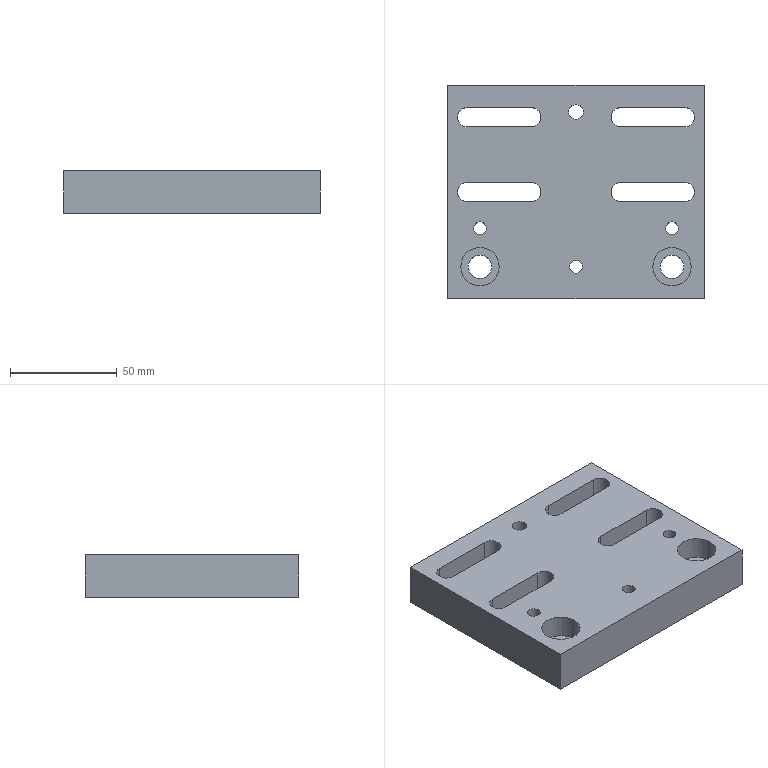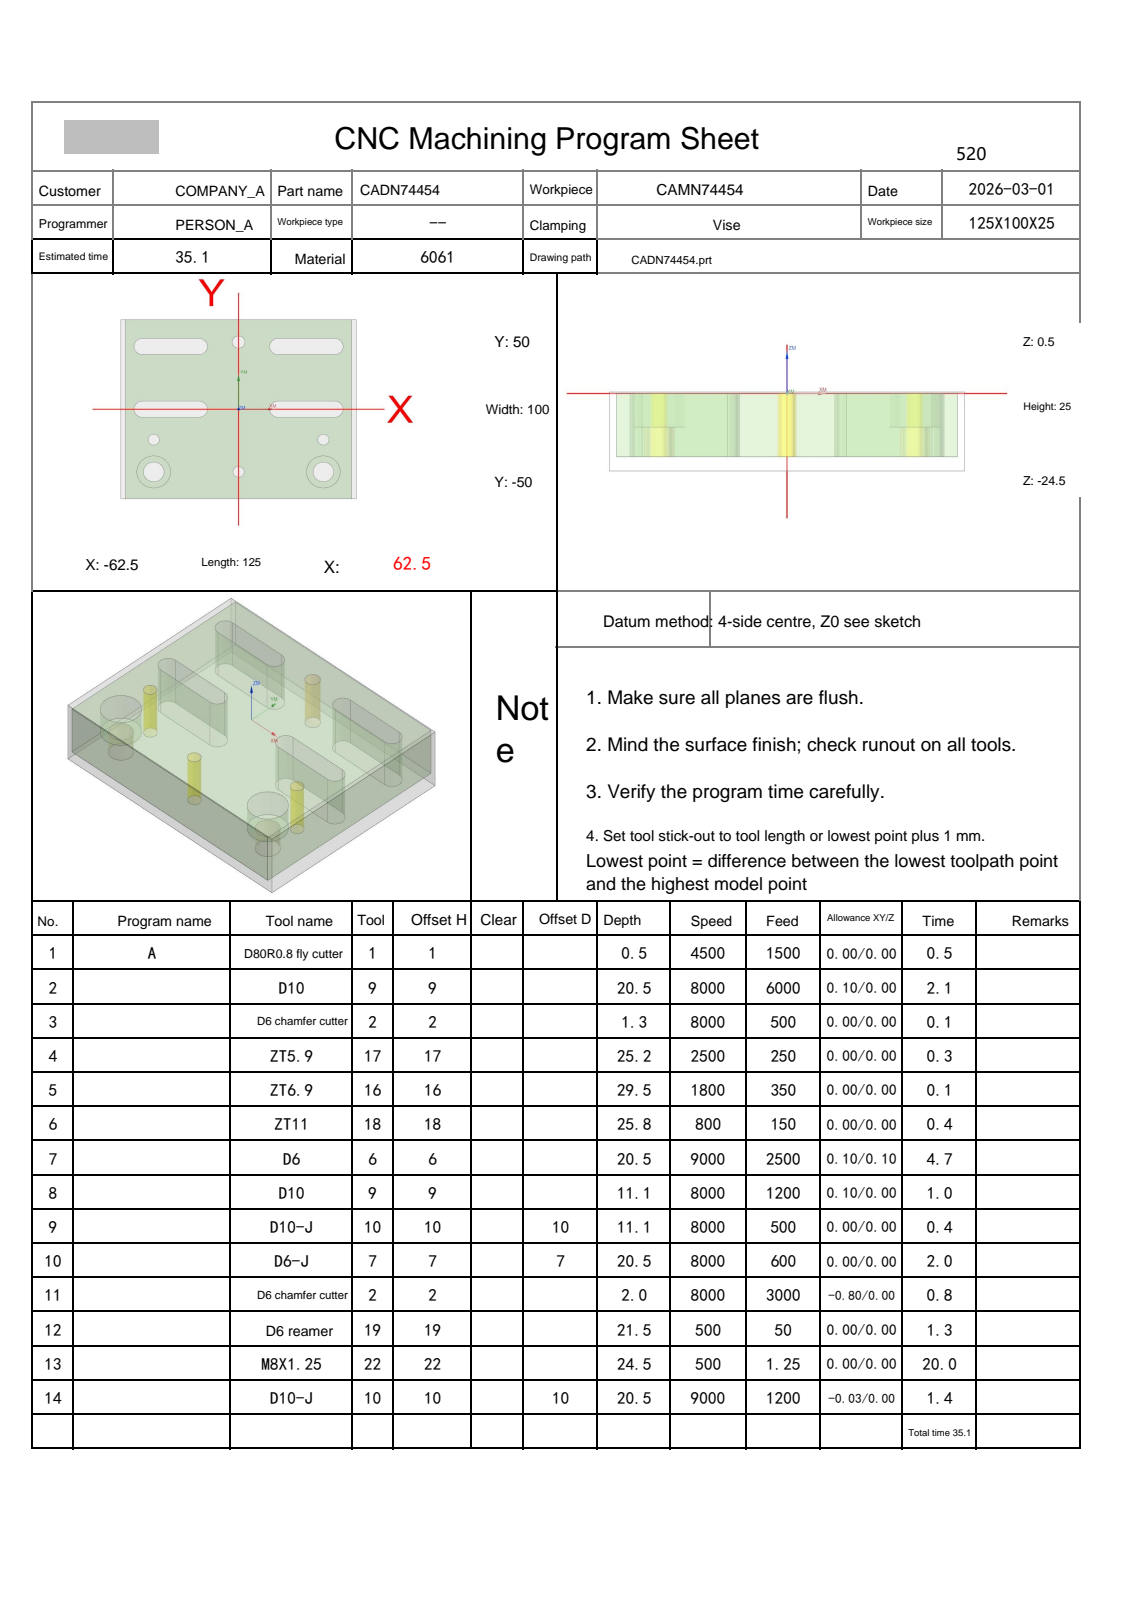NC program | NX | posted by the shop | part box 120 x 100 x 20 mm
Lines 2070 to 2160 of 2160:
N14 T10 M06
(D10-J  D=10. R=0. H=10 ce=0.00 di=0.00)
G00 G90 G54 X-61.013 Y56.116 M03 S9000
G43 H10 Z50.
M08
Z-9.5
G01 Z-10. F1200.
G41 D10
X-60.997 Y55.917
G03 X-60. Y55. I.997 J.083
G01 X60.
G02 X65. Y50. I0.0 J-5.
G01 Y-50.
G02 X60. Y-55. I-5. J0.0
G01 X-60.
G02 X-65. Y-50. I0.0 J5.
G01 Y50.
G02 X-60. Y55. I5. J0.0
G01 X-59.5
G03 X-58.5 Y56. I0.0 J1.
G01 G40 Y56.2
Z-9.5
G00 Z50.
X-61.013 Y56.116
Z-19.5
G01 Z-20.
G41 D10
X-60.997 Y55.917
G03 X-60. Y55. I.997 J.083
G01 X60.
G02 X65. Y50. I0.0 J-5.
G01 Y-50.
G02 X60. Y-55. I-5. J0.0
G01 X-60.
G02 X-65. Y-50. I0.0 J5.
G01 Y50.
G02 X-60. Y55. I5. J0.0
G01 X-59.5
G03 X-58.5 Y56. I0.0 J1.
G01 G40 Y56.2
Z-19.5
G00 Z50.
G00 G90 X66.511 Y-56.399 M03 S8000
Z10.5
Z-8.5
G01 Z-10. F1000.
G41 D10
X66.475 Y-56.202
G03 X65. Y-54.975 I-1.475 J-.273
G01 X-65.
G03 X-66.475 Y-56.202 I0.0 J-1.5
G01 G40 X-66.511 Y-56.399
Z-8.5
G00 X66.511
Z-18.5
G01 Z-20.
G41 D10
X66.475 Y-56.202
G03 X65. Y-54.975 I-1.475 J-.273
G01 X-65.
G03 X-66.475 Y-56.202 I0.0 J-1.5
G01 G40 X-66.511 Y-56.399
Z-18.5
G00 Z10.5
Y56.399
Z-8.5
G01 Z-10.
G41 D10
X-66.475 Y56.202
G03 X-65. Y54.975 I1.475 J.273
G01 X65.
G03 X66.475 Y56.202 I0.0 J1.5
G01 G40 X66.511 Y56.399
Z-8.5
G00 X-66.511
Z-18.5
G01 Z-20.
G41 D10
X-66.475 Y56.202
G03 X-65. Y54.975 I1.475 J.273
G01 X65.
G03 X66.475 Y56.202 I0.0 J1.5
G01 G40 X66.511 Y56.399
Z-18.5
G00 Z10.5
M05
M09
G91 G28 Z0.0
G91 G28 Y0.0
M30
%